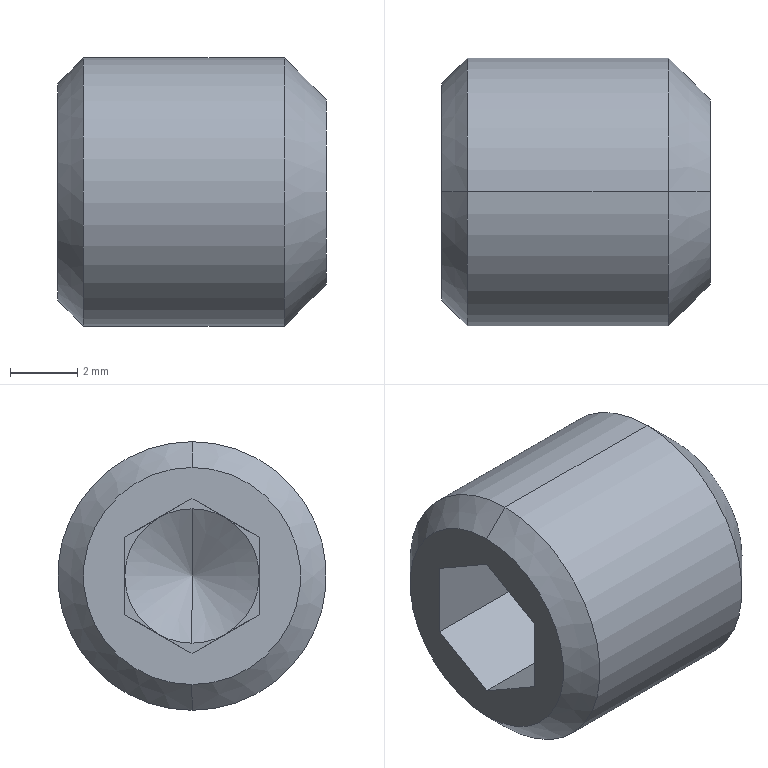Part | STEP file | _SET-SCREW8-8.stp | 1 solid | 22 faces | box 8 x 8 x 8 mm | volume 331.208 mm3 | plane 14 | cone 6 | cylinder 2 | commonest cylinder face diameters 8 x2
STEP:
#1=CARTESIAN_POINT('',(0.,0.,0.));
#2=DIRECTION('',(0.,0.,1.));
#3=DIRECTION('',(1.,0.,0.));
#4=AXIS2_PLACEMENT_3D('',#1,#2,#3);
#5=CARTESIAN_POINT('',(-5.,0.,2.));
#6=VERTEX_POINT('',#5);
#7=CARTESIAN_POINT('',(-5.,-1.,1.732));
#8=VERTEX_POINT('',#7);
#9=CARTESIAN_POINT('',(-5.,0.,0.));
#10=DIRECTION('',(1.,0.,0.));
#11=DIRECTION('',(0.,0.,1.));
#12=AXIS2_PLACEMENT_3D('',#9,#10,#11);
#13=CIRCLE('',#12,2.);
#14=CARTESIAN_POINT('',(-4.845,0.,0.));
#15=DIRECTION('',(-1.,0.,0.));
#16=DIRECTION('',(0.,0.,1.));
#17=AXIS2_PLACEMENT_3D('',#14,#15,#16);
#18=CONICAL_SURFACE('',#17,1.732,1.047);
#19=CARTESIAN_POINT('',(6.283,0.1547));
#20=DIRECTION('',(-1.,0.));
#21=VECTOR('',#20,1.);
#22=LINE('',#19,#21);
#23=(GEOMETRIC_REPRESENTATION_CONTEXT(2)PARAMETRIC_REPRESENTATION_CONTEXT()REPRESENTATION_CONTEXT('',''));
#24=DEFINITIONAL_REPRESENTATION('',(#22),#23);
#25=PCURVE('',#18,#24);
#26=CARTESIAN_POINT('',(-5.,-1.1,1.703));
#27=DIRECTION('',(-1.,0.,0.));
#28=DIRECTION('',(0.,0.,1.));
#29=AXIS2_PLACEMENT_3D('',#26,#27,#28);
#30=PLANE('',#29);
#31=CARTESIAN_POINT('',(0.2968,1.1));
#32=CARTESIAN_POINT('',(0.2968,-2.364));
#33=CARTESIAN_POINT('',(-2.703,-0.6321));
#34=CARTESIAN_POINT('',(-5.703,1.1));
#35=CARTESIAN_POINT('',(-2.703,2.832));
#36=CARTESIAN_POINT('',(0.2968,4.564));
#37=CARTESIAN_POINT('',(0.2968,1.1));
#38=(BOUNDED_CURVE()B_SPLINE_CURVE(2,(#31,#32,#33,#34,#35,#36,#37),.UNSPECIFIED.,.T.,.F.)B_SPLINE_CURVE_WITH_KNOTS((1,2,2,2,2,1),(-2.094,0.,2.094,4.189,6.283,8.378),.UNSPECIFIED.)CURVE()GEOMETRIC_REPRESENTATION_ITEM()RATIONAL_B_SPLINE_CURVE((1.,0.5,1.,0.5,1.,0.5,1.))REPRESENTATION_ITEM(''));
#39=(GEOMETRIC_REPRESENTATION_CONTEXT(2)PARAMETRIC_REPRESENTATION_CONTEXT()REPRESENTATION_CONTEXT('',''));
#40=DEFINITIONAL_REPRESENTATION('',(#38),#39);
#41=PCURVE('',#30,#40);
#42=SURFACE_CURVE('',#13,(#25,#41),.PCURVE_S1.);
#43=EDGE_CURVE('',#6,#8,#42,.T.);
#44=ORIENTED_EDGE('',*,*,#43,.T.);
#45=CARTESIAN_POINT('',(-5.,-2.,0.));
#46=VERTEX_POINT('',#45);
#47=CARTESIAN_POINT('',(-5.,0.,0.));
#48=DIRECTION('',(1.,0.,0.));
#49=DIRECTION('',(0.,0.,1.));
#50=AXIS2_PLACEMENT_3D('',#47,#48,#49);
#51=CIRCLE('',#50,2.);
#52=CARTESIAN_POINT('',(6.283,0.1547));
#53=DIRECTION('',(-1.,0.));
#54=VECTOR('',#53,1.);
#55=LINE('',#52,#54);
#56=(GEOMETRIC_REPRESENTATION_CONTEXT(2)PARAMETRIC_REPRESENTATION_CONTEXT()REPRESENTATION_CONTEXT('',''));
#57=DEFINITIONAL_REPRESENTATION('',(#55),#56);
#58=PCURVE('',#18,#57);
#59=CARTESIAN_POINT('',(-5.,-2.05,-0.0866));
#60=DIRECTION('',(-1.,0.,0.));
#61=DIRECTION('',(0.,0.,1.));
#62=AXIS2_PLACEMENT_3D('',#59,#60,#61);
#63=PLANE('',#62);
#64=CARTESIAN_POINT('',(2.087,2.05));
#65=CARTESIAN_POINT('',(2.087,-1.414));
#66=CARTESIAN_POINT('',(-0.9134,0.3179));
#67=CARTESIAN_POINT('',(-3.913,2.05));
#68=CARTESIAN_POINT('',(-0.9134,3.782));
#69=CARTESIAN_POINT('',(2.087,5.514));
#70=CARTESIAN_POINT('',(2.087,2.05));
#71=(BOUNDED_CURVE()B_SPLINE_CURVE(2,(#64,#65,#66,#67,#68,#69,#70),.UNSPECIFIED.,.T.,.F.)B_SPLINE_CURVE_WITH_KNOTS((1,2,2,2,2,1),(-2.094,0.,2.094,4.189,6.283,8.378),.UNSPECIFIED.)CURVE()GEOMETRIC_REPRESENTATION_ITEM()RATIONAL_B_SPLINE_CURVE((1.,0.5,1.,0.5,1.,0.5,1.))REPRESENTATION_ITEM(''));
#72=(GEOMETRIC_REPRESENTATION_CONTEXT(2)PARAMETRIC_REPRESENTATION_CONTEXT()REPRESENTATION_CONTEXT('',''));
#73=DEFINITIONAL_REPRESENTATION('',(#71),#72);
#74=PCURVE('',#63,#73);
#75=SURFACE_CURVE('',#51,(#58,#74),.PCURVE_S1.);
#76=EDGE_CURVE('',#8,#46,#75,.T.);
#77=ORIENTED_EDGE('',*,*,#76,.T.);
#78=CARTESIAN_POINT('',(-5.,-1.,-1.732));
#79=VERTEX_POINT('',#78);
#80=CARTESIAN_POINT('',(-5.,0.,0.));
#81=DIRECTION('',(1.,0.,0.));
#82=DIRECTION('',(0.,0.,1.));
#83=AXIS2_PLACEMENT_3D('',#80,#81,#82);
#84=CIRCLE('',#83,2.);
#85=CARTESIAN_POINT('',(6.283,0.1547));
#86=DIRECTION('',(-1.,0.));
#87=VECTOR('',#86,1.);
#88=LINE('',#85,#87);
#89=(GEOMETRIC_REPRESENTATION_CONTEXT(2)PARAMETRIC_REPRESENTATION_CONTEXT()REPRESENTATION_CONTEXT('',''));
#90=DEFINITIONAL_REPRESENTATION('',(#88),#89);
#91=PCURVE('',#18,#90);
#92=CARTESIAN_POINT('',(-5.,-2.05,-1.819));
#93=DIRECTION('',(-1.,0.,0.));
#94=DIRECTION('',(0.,0.,1.));
#95=AXIS2_PLACEMENT_3D('',#92,#93,#94);
#96=PLANE('',#95);
#97=CARTESIAN_POINT('',(3.819,2.05));
#98=CARTESIAN_POINT('',(3.819,-1.414));
#99=CARTESIAN_POINT('',(0.8187,0.3179));
#100=CARTESIAN_POINT('',(-2.181,2.05));
#101=CARTESIAN_POINT('',(0.8187,3.782));
#102=CARTESIAN_POINT('',(3.819,5.514));
#103=CARTESIAN_POINT('',(3.819,2.05));
#104=(BOUNDED_CURVE()B_SPLINE_CURVE(2,(#97,#98,#99,#100,#101,#102,#103),.UNSPECIFIED.,.T.,.F.)B_SPLINE_CURVE_WITH_KNOTS((1,2,2,2,2,1),(-2.094,0.,2.094,4.189,6.283,8.378),.UNSPECIFIED.)CURVE()GEOMETRIC_REPRESENTATION_ITEM()RATIONAL_B_SPLINE_CURVE((1.,0.5,1.,0.5,1.,0.5,1.))REPRESENTATION_ITEM(''));
#105=(GEOMETRIC_REPRESENTATION_CONTEXT(2)PARAMETRIC_REPRESENTATION_CONTEXT()REPRESENTATION_CONTEXT('',''));
#106=DEFINITIONAL_REPRESENTATION('',(#104),#105);
#107=PCURVE('',#96,#106);
#108=SURFACE_CURVE('',#84,(#91,#107),.PCURVE_S1.);
#109=EDGE_CURVE('',#46,#79,#108,.T.);
#110=ORIENTED_EDGE('',*,*,#109,.T.);
#111=CARTESIAN_POINT('',(-5.,0.,-2.));
#112=VERTEX_POINT('',#111);
#113=CARTESIAN_POINT('',(-5.,0.,0.));
#114=DIRECTION('',(1.,0.,0.));
#115=DIRECTION('',(0.,0.,1.));
#116=AXIS2_PLACEMENT_3D('',#113,#114,#115);
#117=CIRCLE('',#116,2.);
#118=CARTESIAN_POINT('',(6.283,0.1547));
#119=DIRECTION('',(-1.,0.));
#120=VECTOR('',#119,1.);
#121=LINE('',#118,#120);
#122=(GEOMETRIC_REPRESENTATION_CONTEXT(2)PARAMETRIC_REPRESENTATION_CONTEXT()REPRESENTATION_CONTEXT('',''));
#123=DEFINITIONAL_REPRESENTATION('',(#121),#122);
#124=PCURVE('',#18,#123);
#125=CARTESIAN_POINT('',(-5.,-1.1,-2.338));
#126=DIRECTION('',(-1.,0.,0.));
#127=DIRECTION('',(0.,0.,1.));
#128=AXIS2_PLACEMENT_3D('',#125,#126,#127);
#129=PLANE('',#128);
#130=CARTESIAN_POINT('',(4.338,1.1));
#131=CARTESIAN_POINT('',(4.338,-2.364));
#132=CARTESIAN_POINT('',(1.338,-0.6321));
#133=CARTESIAN_POINT('',(-1.662,1.1));
#134=CARTESIAN_POINT('',(1.338,2.832));
#135=CARTESIAN_POINT('',(4.338,4.564));
#136=CARTESIAN_POINT('',(4.338,1.1));
#137=(BOUNDED_CURVE()B_SPLINE_CURVE(2,(#130,#131,#132,#133,#134,#135,#136),.UNSPECIFIED.,.T.,.F.)B_SPLINE_CURVE_WITH_KNOTS((1,2,2,2,2,1),(-2.094,0.,2.094,4.189,6.283,8.378),.UNSPECIFIED.)CURVE()GEOMETRIC_REPRESENTATION_ITEM()RATIONAL_B_SPLINE_CURVE((1.,0.5,1.,0.5,1.,0.5,1.))REPRESENTATION_ITEM(''));
#138=(GEOMETRIC_REPRESENTATION_CONTEXT(2)PARAMETRIC_REPRESENTATION_CONTEXT()REPRESENTATION_CONTEXT('',''));
#139=DEFINITIONAL_REPRESENTATION('',(#137),#138);
#140=PCURVE('',#129,#139);
#141=SURFACE_CURVE('',#117,(#124,#140),.PCURVE_S1.);
#142=EDGE_CURVE('',#79,#112,#141,.T.);
#143=ORIENTED_EDGE('',*,*,#142,.T.);
#144=CARTESIAN_POINT('',(-3.845,0.,0.));
#145=VERTEX_POINT('',#144);
#146=CARTESIAN_POINT('',(-4.845,0.,-1.732));
#147=DIRECTION('',(-0.5,0.,-0.866));
#148=VECTOR('',#147,1.);
#149=LINE('',#146,#148);
#150=CARTESIAN_POINT('',(3.142,0.));
#151=DIRECTION('',(0.,1.));
#152=VECTOR('',#151,1.);
#153=LINE('',#150,#152);
#154=(GEOMETRIC_REPRESENTATION_CONTEXT(2)PARAMETRIC_REPRESENTATION_CONTEXT()REPRESENTATION_CONTEXT('',''));
#155=DEFINITIONAL_REPRESENTATION('',(#153),#154);
#156=PCURVE('',#18,#155);
#157=CARTESIAN_POINT('',(-4.845,0.,0.));
#158=DIRECTION('',(-1.,0.,0.));
#159=DIRECTION('',(0.,0.,1.));
#160=AXIS2_PLACEMENT_3D('',#157,#158,#159);
#161=CONICAL_SURFACE('',#160,1.732,1.047);
#162=CARTESIAN_POINT('',(3.142,0.));
#163=DIRECTION('',(0.,1.));
#164=VECTOR('',#163,1.);
#165=LINE('',#162,#164);
#166=(GEOMETRIC_REPRESENTATION_CONTEXT(2)PARAMETRIC_REPRESENTATION_CONTEXT()REPRESENTATION_CONTEXT('',''));
#167=DEFINITIONAL_REPRESENTATION('',(#165),#166);
#168=PCURVE('',#161,#167);
#169=SURFACE_CURVE('',#149,(#156,#168),.PCURVE_S1.);
#170=EDGE_CURVE('',#145,#112,#169,.T.);
#171=ORIENTED_EDGE('',*,*,#170,.F.);
#172=CARTESIAN_POINT('',(-4.845,0.,1.732));
#173=DIRECTION('',(-0.5,0.,0.866));
#174=VECTOR('',#173,1.);
#175=LINE('',#172,#174);
#176=CARTESIAN_POINT('',(6.283,0.));
#177=DIRECTION('',(0.,1.));
#178=VECTOR('',#177,1.);
#179=LINE('',#176,#178);
#180=(GEOMETRIC_REPRESENTATION_CONTEXT(2)PARAMETRIC_REPRESENTATION_CONTEXT()REPRESENTATION_CONTEXT('',''));
#181=DEFINITIONAL_REPRESENTATION('',(#179),#180);
#182=PCURVE('',#18,#181);
#183=CARTESIAN_POINT('',(0.,0.));
#184=DIRECTION('',(0.,1.));
#185=VECTOR('',#184,1.);
#186=LINE('',#183,#185);
#187=(GEOMETRIC_REPRESENTATION_CONTEXT(2)PARAMETRIC_REPRESENTATION_CONTEXT()REPRESENTATION_CONTEXT('',''));
#188=DEFINITIONAL_REPRESENTATION('',(#186),#187);
#189=PCURVE('',#161,#188);
#190=SURFACE_CURVE('',#175,(#182,#189),.PCURVE_S1.);
#191=EDGE_CURVE('',#145,#6,#190,.T.);
#192=ORIENTED_EDGE('',*,*,#191,.T.);
#193=EDGE_LOOP('',(#44,#77,#110,#143,#171,#192));
#194=FACE_BOUND('',#193,.F.);
#195=ADVANCED_FACE('',(#194),#18,.F.);
#196=CARTESIAN_POINT('',(-8.,2.,-1.155));
#197=VERTEX_POINT('',#196);
#198=CARTESIAN_POINT('',(-8.,0.,-2.309));
#199=VERTEX_POINT('',#198);
#200=CARTESIAN_POINT('',(-8.,2.,-1.155));
#201=DIRECTION('',(0.,-0.866,-0.5));
#202=VECTOR('',#201,1.);
#203=LINE('',#200,#202);
#204=CARTESIAN_POINT('',(-8.15,-0.1,-2.367));
#205=DIRECTION('',(0.,0.5,-0.866));
#206=DIRECTION('',(-1.,0.,0.));
#207=AXIS2_PLACEMENT_3D('',#204,#205,#206);
#208=PLANE('',#207);
#209=CARTESIAN_POINT('',(-0.15,2.425));
#210=DIRECTION('',(0.,-1.));
#211=VECTOR('',#210,1.);
#212=LINE('',#209,#211);
#213=(GEOMETRIC_REPRESENTATION_CONTEXT(2)PARAMETRIC_REPRESENTATION_CONTEXT()REPRESENTATION_CONTEXT('',''));
#214=DEFINITIONAL_REPRESENTATION('',(#212),#213);
#215=PCURVE('',#208,#214);
#216=CARTESIAN_POINT('',(-8.,-3.556,3.556));
#217=DIRECTION('',(1.,0.,0.));
#218=DIRECTION('',(0.,1.,0.));
#219=AXIS2_PLACEMENT_3D('',#216,#217,#218);
#220=PLANE('',#219);
#221=CARTESIAN_POINT('',(5.556,-4.711));
#222=DIRECTION('',(-0.866,-0.5));
#223=VECTOR('',#222,1.);
#224=LINE('',#221,#223);
#225=(GEOMETRIC_REPRESENTATION_CONTEXT(2)PARAMETRIC_REPRESENTATION_CONTEXT()REPRESENTATION_CONTEXT('',''));
#226=DEFINITIONAL_REPRESENTATION('',(#224),#225);
#227=PCURVE('',#220,#226);
#228=SURFACE_CURVE('',#203,(#215,#227),.PCURVE_S1.);
#229=EDGE_CURVE('',#197,#199,#228,.T.);
#230=ORIENTED_EDGE('',*,*,#229,.T.);
#231=CARTESIAN_POINT('',(-5.,0.,-2.309));
#232=VERTEX_POINT('',#231);
#233=CARTESIAN_POINT('',(-5.,0.,-2.309));
#234=DIRECTION('',(-1.,0.,0.));
#235=VECTOR('',#234,1.);
#236=LINE('',#233,#235);
#237=CARTESIAN_POINT('',(-3.15,0.1155));
#238=DIRECTION('',(1.,0.));
#239=VECTOR('',#238,1.);
#240=LINE('',#237,#239);
#241=(GEOMETRIC_REPRESENTATION_CONTEXT(2)PARAMETRIC_REPRESENTATION_CONTEXT()REPRESENTATION_CONTEXT('',''));
#242=DEFINITIONAL_REPRESENTATION('',(#240),#241);
#243=PCURVE('',#208,#242);
#244=CARTESIAN_POINT('',(-8.15,-2.1,-1.097));
#245=DIRECTION('',(0.,-0.5,-0.866));
#246=DIRECTION('',(0.,-0.866,0.5));
#247=AXIS2_PLACEMENT_3D('',#244,#245,#246);
#248=PLANE('',#247);
#249=CARTESIAN_POINT('',(-2.425,-3.15));
#250=DIRECTION('',(0.,1.));
#251=VECTOR('',#250,1.);
#252=LINE('',#249,#251);
#253=(GEOMETRIC_REPRESENTATION_CONTEXT(2)PARAMETRIC_REPRESENTATION_CONTEXT()REPRESENTATION_CONTEXT('',''));
#254=DEFINITIONAL_REPRESENTATION('',(#252),#253);
#255=PCURVE('',#248,#254);
#256=SURFACE_CURVE('',#236,(#243,#255),.PCURVE_S1.);
#257=EDGE_CURVE('',#232,#199,#256,.T.);
#258=ORIENTED_EDGE('',*,*,#257,.F.);
#259=CARTESIAN_POINT('',(-5.,1.,-1.732));
#260=VERTEX_POINT('',#259);
#261=CARTESIAN_POINT('',(-5.,1.,-1.732));
#262=DIRECTION('',(0.,-0.866,-0.5));
#263=VECTOR('',#262,1.);
#264=LINE('',#261,#263);
#265=CARTESIAN_POINT('',(-3.15,1.27));
#266=DIRECTION('',(0.,-1.));
#267=VECTOR('',#266,1.);
#268=LINE('',#265,#267);
#269=(GEOMETRIC_REPRESENTATION_CONTEXT(2)PARAMETRIC_REPRESENTATION_CONTEXT()REPRESENTATION_CONTEXT('',''));
#270=DEFINITIONAL_REPRESENTATION('',(#268),#269);
#271=PCURVE('',#208,#270);
#272=CARTESIAN_POINT('',(0.6062,2.1));
#273=DIRECTION('',(-0.5,-0.866));
#274=VECTOR('',#273,1.);
#275=LINE('',#272,#274);
#276=(GEOMETRIC_REPRESENTATION_CONTEXT(2)PARAMETRIC_REPRESENTATION_CONTEXT()REPRESENTATION_CONTEXT('',''));
#277=DEFINITIONAL_REPRESENTATION('',(#275),#276);
#278=PCURVE('',#129,#277);
#279=SURFACE_CURVE('',#264,(#271,#278),.PCURVE_S1.);
#280=EDGE_CURVE('',#260,#232,#279,.T.);
#281=ORIENTED_EDGE('',*,*,#280,.F.);
#282=CARTESIAN_POINT('',(-5.,2.,-1.155));
#283=VERTEX_POINT('',#282);
#284=CARTESIAN_POINT('',(-5.,2.,-1.155));
#285=DIRECTION('',(0.,-0.866,-0.5));
#286=VECTOR('',#285,1.);
#287=LINE('',#284,#286);
#288=CARTESIAN_POINT('',(-3.15,2.425));
#289=DIRECTION('',(0.,-1.));
#290=VECTOR('',#289,1.);
#291=LINE('',#288,#290);
#292=(GEOMETRIC_REPRESENTATION_CONTEXT(2)PARAMETRIC_REPRESENTATION_CONTEXT()REPRESENTATION_CONTEXT('',''));
#293=DEFINITIONAL_REPRESENTATION('',(#291),#292);
#294=PCURVE('',#208,#293);
#295=CARTESIAN_POINT('',(-5.,0.95,-1.819));
#296=DIRECTION('',(-1.,0.,0.));
#297=DIRECTION('',(0.,0.,1.));
#298=AXIS2_PLACEMENT_3D('',#295,#296,#297);
#299=PLANE('',#298);
#300=CARTESIAN_POINT('',(0.664,1.05));
#301=DIRECTION('',(-0.5,-0.866));
#302=VECTOR('',#301,1.);
#303=LINE('',#300,#302);
#304=(GEOMETRIC_REPRESENTATION_CONTEXT(2)PARAMETRIC_REPRESENTATION_CONTEXT()REPRESENTATION_CONTEXT('',''));
#305=DEFINITIONAL_REPRESENTATION('',(#303),#304);
#306=PCURVE('',#299,#305);
#307=SURFACE_CURVE('',#287,(#294,#306),.PCURVE_S1.);
#308=EDGE_CURVE('',#283,#260,#307,.T.);
#309=ORIENTED_EDGE('',*,*,#308,.F.);
#310=CARTESIAN_POINT('',(-5.,2.,-1.155));
#311=DIRECTION('',(-1.,0.,0.));
#312=VECTOR('',#311,1.);
#313=LINE('',#310,#312);
#314=CARTESIAN_POINT('',(-3.15,2.425));
#315=DIRECTION('',(1.,0.));
#316=VECTOR('',#315,1.);
#317=LINE('',#314,#316);
#318=(GEOMETRIC_REPRESENTATION_CONTEXT(2)PARAMETRIC_REPRESENTATION_CONTEXT()REPRESENTATION_CONTEXT('',''));
#319=DEFINITIONAL_REPRESENTATION('',(#317),#318);
#320=PCURVE('',#208,#319);
#321=CARTESIAN_POINT('',(-8.15,2.,-1.27));
#322=DIRECTION('',(0.,1.,0.));
#323=DIRECTION('',(1.,0.,0.));
#324=AXIS2_PLACEMENT_3D('',#321,#322,#323);
#325=PLANE('',#324);
#326=CARTESIAN_POINT('',(3.15,-0.1155));
#327=DIRECTION('',(-1.,0.));
#328=VECTOR('',#327,1.);
#329=LINE('',#326,#328);
#330=(GEOMETRIC_REPRESENTATION_CONTEXT(2)PARAMETRIC_REPRESENTATION_CONTEXT()REPRESENTATION_CONTEXT('',''));
#331=DEFINITIONAL_REPRESENTATION('',(#329),#330);
#332=PCURVE('',#325,#331);
#333=SURFACE_CURVE('',#313,(#320,#332),.PCURVE_S1.);
#334=EDGE_CURVE('',#283,#197,#333,.T.);
#335=ORIENTED_EDGE('',*,*,#334,.T.);
#336=EDGE_LOOP('',(#230,#258,#281,#309,#335));
#337=FACE_BOUND('',#336,.T.);
#338=ADVANCED_FACE('',(#337),#208,.F.);
#339=CARTESIAN_POINT('',(-5.,2.,1.155));
#340=VERTEX_POINT('',#339);
#341=CARTESIAN_POINT('',(-8.,2.,1.155));
#342=VERTEX_POINT('',#341);
#343=CARTESIAN_POINT('',(-5.,2.,1.155));
#344=DIRECTION('',(-1.,0.,0.));
#345=VECTOR('',#344,1.);
#346=LINE('',#343,#345);
#347=CARTESIAN_POINT('',(3.15,-2.425));
#348=DIRECTION('',(-1.,0.));
#349=VECTOR('',#348,1.);
#350=LINE('',#347,#349);
#351=(GEOMETRIC_REPRESENTATION_CONTEXT(2)PARAMETRIC_REPRESENTATION_CONTEXT()REPRESENTATION_CONTEXT('',''));
#352=DEFINITIONAL_REPRESENTATION('',(#350),#351);
#353=PCURVE('',#325,#352);
#354=CARTESIAN_POINT('',(-8.15,2.1,1.097));
#355=DIRECTION('',(0.,0.5,0.866));
#356=DIRECTION('',(1.,0.,0.));
#357=AXIS2_PLACEMENT_3D('',#354,#355,#356);
#358=PLANE('',#357);
#359=CARTESIAN_POINT('',(3.15,-0.1155));
#360=DIRECTION('',(-1.,0.));
#361=VECTOR('',#360,1.);
#362=LINE('',#359,#361);
#363=(GEOMETRIC_REPRESENTATION_CONTEXT(2)PARAMETRIC_REPRESENTATION_CONTEXT()REPRESENTATION_CONTEXT('',''));
#364=DEFINITIONAL_REPRESENTATION('',(#362),#363);
#365=PCURVE('',#358,#364);
#366=SURFACE_CURVE('',#346,(#353,#365),.PCURVE_S1.);
#367=EDGE_CURVE('',#340,#342,#366,.T.);
#368=ORIENTED_EDGE('',*,*,#367,.T.);
#369=CARTESIAN_POINT('',(-8.,2.,-1.155));
#370=DIRECTION('',(0.,0.,1.));
#371=VECTOR('',#370,1.);
#372=LINE('',#369,#371);
#373=CARTESIAN_POINT('',(0.15,-0.1155));
#374=DIRECTION('',(0.,-1.));
#375=VECTOR('',#374,1.);
#376=LINE('',#373,#375);
#377=(GEOMETRIC_REPRESENTATION_CONTEXT(2)PARAMETRIC_REPRESENTATION_CONTEXT()REPRESENTATION_CONTEXT('',''));
#378=DEFINITIONAL_REPRESENTATION('',(#376),#377);
#379=PCURVE('',#325,#378);
#380=CARTESIAN_POINT('',(5.556,-4.711));
#381=DIRECTION('',(0.,1.));
#382=VECTOR('',#381,1.);
#383=LINE('',#380,#382);
#384=(GEOMETRIC_REPRESENTATION_CONTEXT(2)PARAMETRIC_REPRESENTATION_CONTEXT()REPRESENTATION_CONTEXT('',''));
#385=DEFINITIONAL_REPRESENTATION('',(#383),#384);
#386=PCURVE('',#220,#385);
#387=SURFACE_CURVE('',#372,(#379,#386),.PCURVE_S1.);
#388=EDGE_CURVE('',#197,#342,#387,.T.);
#389=ORIENTED_EDGE('',*,*,#388,.F.);
#390=ORIENTED_EDGE('',*,*,#334,.F.);
#391=CARTESIAN_POINT('',(-5.,2.,0.));
#392=VERTEX_POINT('',#391);
#393=CARTESIAN_POINT('',(-5.,2.,0.));
#394=DIRECTION('',(0.,0.,-1.));
#395=VECTOR('',#394,1.);
#396=LINE('',#393,#395);
#397=CARTESIAN_POINT('',(3.15,-1.27));
#398=DIRECTION('',(0.,1.));
#399=VECTOR('',#398,1.);
#400=LINE('',#397,#399);
#401=(GEOMETRIC_REPRESENTATION_CONTEXT(2)PARAMETRIC_REPRESENTATION_CONTEXT()REPRESENTATION_CONTEXT('',''));
#402=DEFINITIONAL_REPRESENTATION('',(#400),#401);
#403=PCURVE('',#325,#402);
#404=CARTESIAN_POINT('',(1.819,1.05));
#405=DIRECTION('',(-1.,0.));
#406=VECTOR('',#405,1.);
#407=LINE('',#404,#406);
#408=(GEOMETRIC_REPRESENTATION_CONTEXT(2)PARAMETRIC_REPRESENTATION_CONTEXT()REPRESENTATION_CONTEXT('',''));
#409=DEFINITIONAL_REPRESENTATION('',(#407),#408);
#410=PCURVE('',#299,#409);
#411=SURFACE_CURVE('',#396,(#403,#410),.PCURVE_S1.);
#412=EDGE_CURVE('',#392,#283,#411,.T.);
#413=ORIENTED_EDGE('',*,*,#412,.F.);
#414=CARTESIAN_POINT('',(-5.,2.,1.155));
#415=DIRECTION('',(0.,0.,-1.));
#416=VECTOR('',#415,1.);
#417=LINE('',#414,#416);
#418=CARTESIAN_POINT('',(3.15,-2.425));
#419=DIRECTION('',(0.,1.));
#420=VECTOR('',#419,1.);
#421=LINE('',#418,#420);
#422=(GEOMETRIC_REPRESENTATION_CONTEXT(2)PARAMETRIC_REPRESENTATION_CONTEXT()REPRESENTATION_CONTEXT('',''));
#423=DEFINITIONAL_REPRESENTATION('',(#421),#422);
#424=PCURVE('',#325,#423);
#425=CARTESIAN_POINT('',(-5.,0.95,-0.0866));
#426=DIRECTION('',(-1.,0.,0.));
#427=DIRECTION('',(0.,0.,1.));
#428=AXIS2_PLACEMENT_3D('',#425,#426,#427);
#429=PLANE('',#428);
#430=CARTESIAN_POINT('',(1.241,1.05));
#431=DIRECTION('',(-1.,0.));
#432=VECTOR('',#431,1.);
#433=LINE('',#430,#432);
#434=(GEOMETRIC_REPRESENTATION_CONTEXT(2)PARAMETRIC_REPRESENTATION_CONTEXT()REPRESENTATION_CONTEXT('',''));
#435=DEFINITIONAL_REPRESENTATION('',(#433),#434);
#436=PCURVE('',#429,#435);
#437=SURFACE_CURVE('',#417,(#424,#436),.PCURVE_S1.);
#438=EDGE_CURVE('',#340,#392,#437,.T.);
#439=ORIENTED_EDGE('',*,*,#438,.F.);
#440=EDGE_LOOP('',(#368,#389,#390,#413,#439));
#441=FACE_BOUND('',#440,.T.);
#442=ADVANCED_FACE('',(#441),#325,.F.);
#443=CARTESIAN_POINT('',(-8.,0.,2.309));
#444=VERTEX_POINT('',#443);
#445=CARTESIAN_POINT('',(-8.,0.,2.309));
#446=DIRECTION('',(0.,0.866,-0.5));
#447=VECTOR('',#446,1.);
#448=LINE('',#445,#447);
#449=CARTESIAN_POINT('',(0.15,-2.425));
#450=DIRECTION('',(0.,1.));
#451=VECTOR('',#450,1.);
#452=LINE('',#449,#451);
#453=(GEOMETRIC_REPRESENTATION_CONTEXT(2)PARAMETRIC_REPRESENTATION_CONTEXT()REPRESENTATION_CONTEXT('',''));
#454=DEFINITIONAL_REPRESENTATION('',(#452),#453);
#455=PCURVE('',#358,#454);
#456=CARTESIAN_POINT('',(3.556,-1.247));
#457=DIRECTION('',(0.866,-0.5));
#458=VECTOR('',#457,1.);
#459=LINE('',#456,#458);
#460=(GEOMETRIC_REPRESENTATION_CONTEXT(2)PARAMETRIC_REPRESENTATION_CONTEXT()REPRESENTATION_CONTEXT('',''));
#461=DEFINITIONAL_REPRESENTATION('',(#459),#460);
#462=PCURVE('',#220,#461);
#463=SURFACE_CURVE('',#448,(#455,#462),.PCURVE_S1.);
#464=EDGE_CURVE('',#444,#342,#463,.T.);
#465=ORIENTED_EDGE('',*,*,#464,.T.);
#466=ORIENTED_EDGE('',*,*,#367,.F.);
#467=CARTESIAN_POINT('',(-5.,1.,1.732));
#468=VERTEX_POINT('',#467);
#469=CARTESIAN_POINT('',(-5.,1.,1.732));
#470=DIRECTION('',(0.,0.866,-0.5));
#471=VECTOR('',#470,1.);
#472=LINE('',#469,#471);
#473=CARTESIAN_POINT('',(3.15,-1.27));
#474=DIRECTION('',(0.,1.));
#475=VECTOR('',#474,1.);
#476=LINE('',#473,#475);
#477=(GEOMETRIC_REPRESENTATION_CONTEXT(2)PARAMETRIC_REPRESENTATION_CONTEXT()REPRESENTATION_CONTEXT('',''));
#478=DEFINITIONAL_REPRESENTATION('',(#476),#477);
#479=PCURVE('',#358,#478);
#480=CARTESIAN_POINT('',(1.819,0.05));
#481=DIRECTION('',(-0.5,0.866));
#482=VECTOR('',#481,1.);
#483=LINE('',#480,#482);
#484=(GEOMETRIC_REPRESENTATION_CONTEXT(2)PARAMETRIC_REPRESENTATION_CONTEXT()REPRESENTATION_CONTEXT('',''));
#485=DEFINITIONAL_REPRESENTATION('',(#483),#484);
#486=PCURVE('',#429,#485);
#487=SURFACE_CURVE('',#472,(#479,#486),.PCURVE_S1.);
#488=EDGE_CURVE('',#468,#340,#487,.T.);
#489=ORIENTED_EDGE('',*,*,#488,.F.);
#490=CARTESIAN_POINT('',(-5.,0.,2.309));
#491=VERTEX_POINT('',#490);
#492=CARTESIAN_POINT('',(-5.,0.,2.309));
#493=DIRECTION('',(0.,0.866,-0.5));
#494=VECTOR('',#493,1.);
#495=LINE('',#492,#494);
#496=CARTESIAN_POINT('',(3.15,-2.425));
#497=DIRECTION('',(0.,1.));
#498=VECTOR('',#497,1.);
#499=LINE('',#496,#498);
#500=(GEOMETRIC_REPRESENTATION_CONTEXT(2)PARAMETRIC_REPRESENTATION_CONTEXT()REPRESENTATION_CONTEXT('',''));
#501=DEFINITIONAL_REPRESENTATION('',(#499),#500);
#502=PCURVE('',#358,#501);
#503=CARTESIAN_POINT('',(0.6062,1.1));
#504=DIRECTION('',(-0.5,0.866));
#505=VECTOR('',#504,1.);
#506=LINE('',#503,#505);
#507=(GEOMETRIC_REPRESENTATION_CONTEXT(2)PARAMETRIC_REPRESENTATION_CONTEXT()REPRESENTATION_CONTEXT('',''));
#508=DEFINITIONAL_REPRESENTATION('',(#506),#507);
#509=PCURVE('',#30,#508);
#510=SURFACE_CURVE('',#495,(#502,#509),.PCURVE_S1.);
#511=EDGE_CURVE('',#491,#468,#510,.T.);
#512=ORIENTED_EDGE('',*,*,#511,.F.);
#513=CARTESIAN_POINT('',(-5.,0.,2.309));
#514=DIRECTION('',(-1.,0.,0.));
#515=VECTOR('',#514,1.);
#516=LINE('',#513,#515);
#517=CARTESIAN_POINT('',(3.15,-2.425));
#518=DIRECTION('',(-1.,0.));
#519=VECTOR('',#518,1.);
#520=LINE('',#517,#519);
#521=(GEOMETRIC_REPRESENTATION_CONTEXT(2)PARAMETRIC_REPRESENTATION_CONTEXT()REPRESENTATION_CONTEXT('',''));
#522=DEFINITIONAL_REPRESENTATION('',(#520),#521);
#523=PCURVE('',#358,#522);
#524=CARTESIAN_POINT('',(-8.15,0.1,2.367));
#525=DIRECTION('',(0.,-0.5,0.866));
#526=DIRECTION('',(-1.,0.,0.));
#527=AXIS2_PLACEMENT_3D('',#524,#525,#526);
#528=PLANE('',#527);
#529=CARTESIAN_POINT('',(-3.15,0.1155));
#530=DIRECTION('',(1.,0.));
#531=VECTOR('',#530,1.);
#532=LINE('',#529,#531);
#533=(GEOMETRIC_REPRESENTATION_CONTEXT(2)PARAMETRIC_REPRESENTATION_CONTEXT()REPRESENTATION_CONTEXT('',''));
#534=DEFINITIONAL_REPRESENTATION('',(#532),#533);
#535=PCURVE('',#528,#534);
#536=SURFACE_CURVE('',#516,(#523,#535),.PCURVE_S1.);
#537=EDGE_CURVE('',#491,#444,#536,.T.);
#538=ORIENTED_EDGE('',*,*,#537,.T.);
#539=EDGE_LOOP('',(#465,#466,#489,#512,#538));
#540=FACE_BOUND('',#539,.T.);
#541=ADVANCED_FACE('',(#540),#358,.F.);
#542=CARTESIAN_POINT('',(-8.,-2.,1.155));
#543=VERTEX_POINT('',#542);
#544=CARTESIAN_POINT('',(-8.,-2.,1.155));
#545=DIRECTION('',(0.,0.866,0.5));
#546=VECTOR('',#545,1.);
#547=LINE('',#544,#546);
#548=CARTESIAN_POINT('',(-0.15,2.425));
#549=DIRECTION('',(0.,-1.));
#550=VECTOR('',#549,1.);
#551=LINE('',#548,#550);
#552=(GEOMETRIC_REPRESENTATION_CONTEXT(2)PARAMETRIC_REPRESENTATION_CONTEXT()REPRESENTATION_CONTEXT('',''));
#553=DEFINITIONAL_REPRESENTATION('',(#551),#552);
#554=PCURVE('',#528,#553);
#555=CARTESIAN_POINT('',(1.556,-2.402));
#556=DIRECTION('',(0.866,0.5));
#557=VECTOR('',#556,1.);
#558=LINE('',#555,#557);
#559=(GEOMETRIC_REPRESENTATION_CONTEXT(2)PARAMETRIC_REPRESENTATION_CONTEXT()REPRESENTATION_CONTEXT('',''));
#560=DEFINITIONAL_REPRESENTATION('',(#558),#559);
#561=PCURVE('',#220,#560);
#562=SURFACE_CURVE('',#547,(#554,#561),.PCURVE_S1.);
#563=EDGE_CURVE('',#543,#444,#562,.T.);
#564=ORIENTED_EDGE('',*,*,#563,.T.);
#565=ORIENTED_EDGE('',*,*,#537,.F.);
#566=CARTESIAN_POINT('',(-5.,-1.,1.732));
#567=DIRECTION('',(0.,0.866,0.5));
#568=VECTOR('',#567,1.);
#569=LINE('',#566,#568);
#570=CARTESIAN_POINT('',(-3.15,1.27));
#571=DIRECTION('',(0.,-1.));
#572=VECTOR('',#571,1.);
#573=LINE('',#570,#572);
#574=(GEOMETRIC_REPRESENTATION_CONTEXT(2)PARAMETRIC_REPRESENTATION_CONTEXT()REPRESENTATION_CONTEXT('',''));
#575=DEFINITIONAL_REPRESENTATION('',(#573),#574);
#576=PCURVE('',#528,#575);
#577=CARTESIAN_POINT('',(0.02887,0.1));
#578=DIRECTION('',(0.5,0.866));
#579=VECTOR('',#578,1.);
#580=LINE('',#577,#579);
#581=(GEOMETRIC_REPRESENTATION_CONTEXT(2)PARAMETRIC_REPRESENTATION_CONTEXT()REPRESENTATION_CONTEXT('',''));
#582=DEFINITIONAL_REPRESENTATION('',(#580),#581);
#583=PCURVE('',#30,#582);
#584=SURFACE_CURVE('',#569,(#576,#583),.PCURVE_S1.);
#585=EDGE_CURVE('',#8,#491,#584,.T.);
#586=ORIENTED_EDGE('',*,*,#585,.F.);
#587=CARTESIAN_POINT('',(-5.,-2.,1.155));
#588=VERTEX_POINT('',#587);
#589=CARTESIAN_POINT('',(-5.,-2.,1.155));
#590=DIRECTION('',(0.,0.866,0.5));
#591=VECTOR('',#590,1.);
#592=LINE('',#589,#591);
#593=CARTESIAN_POINT('',(-3.15,2.425));
#594=DIRECTION('',(0.,-1.));
#595=VECTOR('',#594,1.);
#596=LINE('',#593,#595);
#597=(GEOMETRIC_REPRESENTATION_CONTEXT(2)PARAMETRIC_REPRESENTATION_CONTEXT()REPRESENTATION_CONTEXT('',''));
#598=DEFINITIONAL_REPRESENTATION('',(#596),#597);
#599=PCURVE('',#528,#598);
#600=CARTESIAN_POINT('',(1.241,0.05));
#601=DIRECTION('',(0.5,0.866));
#602=VECTOR('',#601,1.);
#603=LINE('',#600,#602);
#604=(GEOMETRIC_REPRESENTATION_CONTEXT(2)PARAMETRIC_REPRESENTATION_CONTEXT()REPRESENTATION_CONTEXT('',''));
#605=DEFINITIONAL_REPRESENTATION('',(#603),#604);
#606=PCURVE('',#63,#605);
#607=SURFACE_CURVE('',#592,(#599,#606),.PCURVE_S1.);
#608=EDGE_CURVE('',#588,#8,#607,.T.);
#609=ORIENTED_EDGE('',*,*,#608,.F.);
#610=CARTESIAN_POINT('',(-5.,-2.,1.155));
#611=DIRECTION('',(-1.,0.,0.));
#612=VECTOR('',#611,1.);
#613=LINE('',#610,#612);
#614=CARTESIAN_POINT('',(-3.15,2.425));
#615=DIRECTION('',(1.,0.));
#616=VECTOR('',#615,1.);
#617=LINE('',#614,#616);
#618=(GEOMETRIC_REPRESENTATION_CONTEXT(2)PARAMETRIC_REPRESENTATION_CONTEXT()REPRESENTATION_CONTEXT('',''));
#619=DEFINITIONAL_REPRESENTATION('',(#617),#618);
#620=PCURVE('',#528,#619);
#621=CARTESIAN_POINT('',(-8.15,-2.,1.27));
#622=DIRECTION('',(0.,-1.,0.));
#623=DIRECTION('',(0.,0.,-1.));
#624=AXIS2_PLACEMENT_3D('',#621,#622,#623);
#625=PLANE('',#624);
#626=CARTESIAN_POINT('',(0.1155,3.15));
#627=DIRECTION('',(0.,-1.));
#628=VECTOR('',#627,1.);
#629=LINE('',#626,#628);
#630=(GEOMETRIC_REPRESENTATION_CONTEXT(2)PARAMETRIC_REPRESENTATION_CONTEXT()REPRESENTATION_CONTEXT('',''));
#631=DEFINITIONAL_REPRESENTATION('',(#629),#630);
#632=PCURVE('',#625,#631);
#633=SURFACE_CURVE('',#613,(#620,#632),.PCURVE_S1.);
#634=EDGE_CURVE('',#588,#543,#633,.T.);
#635=ORIENTED_EDGE('',*,*,#634,.T.);
#636=EDGE_LOOP('',(#564,#565,#586,#609,#635));
#637=FACE_BOUND('',#636,.T.);
#638=ADVANCED_FACE('',(#637),#528,.F.);
#639=CARTESIAN_POINT('',(-8.,-2.,-1.155));
#640=VERTEX_POINT('',#639);
#641=CARTESIAN_POINT('',(-8.,-2.,-1.155));
#642=DIRECTION('',(0.,0.,1.));
#643=VECTOR('',#642,1.);
#644=LINE('',#641,#643);
#645=CARTESIAN_POINT('',(2.425,0.15));
#646=DIRECTION('',(-1.,0.));
#647=VECTOR('',#646,1.);
#648=LINE('',#645,#647);
#649=(GEOMETRIC_REPRESENTATION_CONTEXT(2)PARAMETRIC_REPRESENTATION_CONTEXT()REPRESENTATION_CONTEXT('',''));
#650=DEFINITIONAL_REPRESENTATION('',(#648),#649);
#651=PCURVE('',#625,#650);
#652=CARTESIAN_POINT('',(1.556,-4.711));
#653=DIRECTION('',(0.,1.));
#654=VECTOR('',#653,1.);
#655=LINE('',#652,#654);
#656=(GEOMETRIC_REPRESENTATION_CONTEXT(2)PARAMETRIC_REPRESENTATION_CONTEXT()REPRESENTATION_CONTEXT('',''));
#657=DEFINITIONAL_REPRESENTATION('',(#655),#656);
#658=PCURVE('',#220,#657);
#659=SURFACE_CURVE('',#644,(#651,#658),.PCURVE_S1.);
#660=EDGE_CURVE('',#640,#543,#659,.T.);
#661=ORIENTED_EDGE('',*,*,#660,.T.);
#662=ORIENTED_EDGE('',*,*,#634,.F.);
#663=CARTESIAN_POINT('',(-5.,-2.,0.));
#664=DIRECTION('',(0.,0.,1.));
#665=VECTOR('',#664,1.);
#666=LINE('',#663,#665);
#667=CARTESIAN_POINT('',(1.27,3.15));
#668=DIRECTION('',(-1.,0.));
#669=VECTOR('',#668,1.);
#670=LINE('',#667,#669);
#671=(GEOMETRIC_REPRESENTATION_CONTEXT(2)PARAMETRIC_REPRESENTATION_CONTEXT()REPRESENTATION_CONTEXT('',''));
#672=DEFINITIONAL_REPRESENTATION('',(#670),#671);
#673=PCURVE('',#625,#672);
#674=CARTESIAN_POINT('',(0.0866,0.05));
#675=DIRECTION('',(1.,0.));
#676=VECTOR('',#675,1.);
#677=LINE('',#674,#676);
#678=(GEOMETRIC_REPRESENTATION_CONTEXT(2)PARAMETRIC_REPRESENTATION_CONTEXT()REPRESENTATION_CONTEXT('',''));
#679=DEFINITIONAL_REPRESENTATION('',(#677),#678);
#680=PCURVE('',#63,#679);
#681=SURFACE_CURVE('',#666,(#673,#680),.PCURVE_S1.);
#682=EDGE_CURVE('',#46,#588,#681,.T.);
#683=ORIENTED_EDGE('',*,*,#682,.F.);
#684=CARTESIAN_POINT('',(-5.,-2.,-1.155));
#685=VERTEX_POINT('',#684);
#686=CARTESIAN_POINT('',(-5.,-2.,-1.155));
#687=DIRECTION('',(0.,0.,1.));
#688=VECTOR('',#687,1.);
#689=LINE('',#686,#688);
#690=CARTESIAN_POINT('',(2.425,3.15));
#691=DIRECTION('',(-1.,0.));
#692=VECTOR('',#691,1.);
#693=LINE('',#690,#692);
#694=(GEOMETRIC_REPRESENTATION_CONTEXT(2)PARAMETRIC_REPRESENTATION_CONTEXT()REPRESENTATION_CONTEXT('',''));
#695=DEFINITIONAL_REPRESENTATION('',(#693),#694);
#696=PCURVE('',#625,#695);
#697=CARTESIAN_POINT('',(0.664,0.05));
#698=DIRECTION('',(1.,0.));
#699=VECTOR('',#698,1.);
#700=LINE('',#697,#699);
#701=(GEOMETRIC_REPRESENTATION_CONTEXT(2)PARAMETRIC_REPRESENTATION_CONTEXT()REPRESENTATION_CONTEXT('',''));
#702=DEFINITIONAL_REPRESENTATION('',(#700),#701);
#703=PCURVE('',#96,#702);
#704=SURFACE_CURVE('',#689,(#696,#703),.PCURVE_S1.);
#705=EDGE_CURVE('',#685,#46,#704,.T.);
#706=ORIENTED_EDGE('',*,*,#705,.F.);
#707=CARTESIAN_POINT('',(-5.,-2.,-1.155));
#708=DIRECTION('',(-1.,0.,0.));
#709=VECTOR('',#708,1.);
#710=LINE('',#707,#709);
#711=CARTESIAN_POINT('',(2.425,3.15));
#712=DIRECTION('',(0.,-1.));
#713=VECTOR('',#712,1.);
#714=LINE('',#711,#713);
#715=(GEOMETRIC_REPRESENTATION_CONTEXT(2)PARAMETRIC_REPRESENTATION_CONTEXT()REPRESENTATION_CONTEXT('',''));
#716=DEFINITIONAL_REPRESENTATION('',(#714),#715);
#717=PCURVE('',#625,#716);
#718=CARTESIAN_POINT('',(-0.1155,-3.15));
#719=DIRECTION('',(0.,1.));
#720=VECTOR('',#719,1.);
#721=LINE('',#718,#720);
#722=(GEOMETRIC_REPRESENTATION_CONTEXT(2)PARAMETRIC_REPRESENTATION_CONTEXT()REPRESENTATION_CONTEXT('',''));
#723=DEFINITIONAL_REPRESENTATION('',(#721),#722);
#724=PCURVE('',#248,#723);
#725=SURFACE_CURVE('',#710,(#717,#724),.PCURVE_S1.);
#726=EDGE_CURVE('',#685,#640,#725,.T.);
#727=ORIENTED_EDGE('',*,*,#726,.T.);
#728=EDGE_LOOP('',(#661,#662,#683,#706,#727));
#729=FACE_BOUND('',#728,.T.);
#730=ADVANCED_FACE('',(#729),#625,.F.);
#731=CARTESIAN_POINT('',(0.,0.,-2.75));
#732=VERTEX_POINT('',#731);
#733=CARTESIAN_POINT('',(0.,0.,2.75));
#734=VERTEX_POINT('',#733);
#735=CARTESIAN_POINT('',(0.,0.,0.));
#736=DIRECTION('',(1.,0.,0.));
#737=DIRECTION('',(0.,0.,-1.));
#738=AXIS2_PLACEMENT_3D('',#735,#736,#737);
#739=CIRCLE('',#738,2.75);
#740=CARTESIAN_POINT('',(0.,-3.025,-3.025));
#741=DIRECTION('',(-1.,0.,0.));
#742=DIRECTION('',(0.,0.,1.));
#743=AXIS2_PLACEMENT_3D('',#740,#741,#742);
#744=PLANE('',#743);
#745=CARTESIAN_POINT('',(0.275,3.025));
#746=CARTESIAN_POINT('',(0.275,7.788));
#747=CARTESIAN_POINT('',(4.4,5.407));
#748=CARTESIAN_POINT('',(8.525,3.025));
#749=CARTESIAN_POINT('',(4.4,0.6434));
#750=CARTESIAN_POINT('',(0.275,-1.738));
#751=CARTESIAN_POINT('',(0.275,3.025));
#752=(BOUNDED_CURVE()B_SPLINE_CURVE(2,(#745,#746,#747,#748,#749,#750,#751),.UNSPECIFIED.,.T.,.F.)B_SPLINE_CURVE_WITH_KNOTS((1,2,2,2,2,1),(-2.094,0.,2.094,4.189,6.283,8.378),.UNSPECIFIED.)CURVE()GEOMETRIC_REPRESENTATION_ITEM()RATIONAL_B_SPLINE_CURVE((1.,0.5,1.,0.5,1.,0.5,1.))REPRESENTATION_ITEM(''));
#753=(GEOMETRIC_REPRESENTATION_CONTEXT(2)PARAMETRIC_REPRESENTATION_CONTEXT()REPRESENTATION_CONTEXT('',''));
#754=DEFINITIONAL_REPRESENTATION('',(#752),#753);
#755=PCURVE('',#744,#754);
#756=CARTESIAN_POINT('',(0.0625,0.,0.));
#757=DIRECTION('',(-1.,0.,0.));
#758=DIRECTION('',(0.,0.,1.));
#759=AXIS2_PLACEMENT_3D('',#756,#757,#758);
#760=CONICAL_SURFACE('',#759,2.687,0.7854);
#761=CARTESIAN_POINT('',(3.142,0.0625));
#762=DIRECTION('',(-1.,0.));
#763=VECTOR('',#762,1.);
#764=LINE('',#761,#763);
#765=(GEOMETRIC_REPRESENTATION_CONTEXT(2)PARAMETRIC_REPRESENTATION_CONTEXT()REPRESENTATION_CONTEXT('',''));
#766=DEFINITIONAL_REPRESENTATION('',(#764),#765);
#767=PCURVE('',#760,#766);
#768=SURFACE_CURVE('',#739,(#755,#767),.PCURVE_S1.);
#769=EDGE_CURVE('',#732,#734,#768,.T.);
#770=ORIENTED_EDGE('',*,*,#769,.T.);
#771=CARTESIAN_POINT('',(0.,0.,0.));
#772=DIRECTION('',(1.,0.,0.));
#773=DIRECTION('',(0.,0.,-1.));
#774=AXIS2_PLACEMENT_3D('',#771,#772,#773);
#775=CIRCLE('',#774,2.75);
#776=CARTESIAN_POINT('',(0.275,3.025));
#777=CARTESIAN_POINT('',(0.275,7.788));
#778=CARTESIAN_POINT('',(4.4,5.407));
#779=CARTESIAN_POINT('',(8.525,3.025));
#780=CARTESIAN_POINT('',(4.4,0.6434));
#781=CARTESIAN_POINT('',(0.275,-1.738));
#782=CARTESIAN_POINT('',(0.275,3.025));
#783=(BOUNDED_CURVE()B_SPLINE_CURVE(2,(#776,#777,#778,#779,#780,#781,#782),.UNSPECIFIED.,.T.,.F.)B_SPLINE_CURVE_WITH_KNOTS((1,2,2,2,2,1),(-2.094,0.,2.094,4.189,6.283,8.378),.UNSPECIFIED.)CURVE()GEOMETRIC_REPRESENTATION_ITEM()RATIONAL_B_SPLINE_CURVE((1.,0.5,1.,0.5,1.,0.5,1.))REPRESENTATION_ITEM(''));
#784=(GEOMETRIC_REPRESENTATION_CONTEXT(2)PARAMETRIC_REPRESENTATION_CONTEXT()REPRESENTATION_CONTEXT('',''));
#785=DEFINITIONAL_REPRESENTATION('',(#783),#784);
#786=PCURVE('',#744,#785);
#787=CARTESIAN_POINT('',(0.0625,0.,0.));
#788=DIRECTION('',(-1.,0.,0.));
#789=DIRECTION('',(0.,0.,1.));
#790=AXIS2_PLACEMENT_3D('',#787,#788,#789);
#791=CONICAL_SURFACE('',#790,2.687,0.7854);
#792=CARTESIAN_POINT('',(9.425,0.0625));
#793=DIRECTION('',(-1.,0.));
#794=VECTOR('',#793,1.);
#795=LINE('',#792,#794);
#796=(GEOMETRIC_REPRESENTATION_CONTEXT(2)PARAMETRIC_REPRESENTATION_CONTEXT()REPRESENTATION_CONTEXT('',''));
#797=DEFINITIONAL_REPRESENTATION('',(#795),#796);
#798=PCURVE('',#791,#797);
#799=SURFACE_CURVE('',#775,(#786,#798),.PCURVE_S1.);
#800=EDGE_CURVE('',#734,#732,#799,.T.);
#801=ORIENTED_EDGE('',*,*,#800,.T.);
#802=EDGE_LOOP('',(#770,#801));
#803=FACE_BOUND('',#802,.T.);
#804=ADVANCED_FACE('',(#803),#744,.F.);
#805=CARTESIAN_POINT('',(-1.25,0.,4.));
#806=VERTEX_POINT('',#805);
#807=CARTESIAN_POINT('',(-1.25,0.,4.));
#808=DIRECTION('',(0.7071,0.,-0.7071));
#809=VECTOR('',#808,1.);
#810=LINE('',#807,#809);
#811=CARTESIAN_POINT('',(0.,1.313));
#812=DIRECTION('',(0.,-1.));
#813=VECTOR('',#812,1.);
#814=LINE('',#811,#813);
#815=(GEOMETRIC_REPRESENTATION_CONTEXT(2)PARAMETRIC_REPRESENTATION_CONTEXT()REPRESENTATION_CONTEXT('',''));
#816=DEFINITIONAL_REPRESENTATION('',(#814),#815);
#817=PCURVE('',#760,#816);
#818=CARTESIAN_POINT('',(6.283,1.313));
#819=DIRECTION('',(0.,-1.));
#820=VECTOR('',#819,1.);
#821=LINE('',#818,#820);
#822=(GEOMETRIC_REPRESENTATION_CONTEXT(2)PARAMETRIC_REPRESENTATION_CONTEXT()REPRESENTATION_CONTEXT('',''));
#823=DEFINITIONAL_REPRESENTATION('',(#821),#822);
#824=PCURVE('',#791,#823);
#825=SURFACE_CURVE('',#810,(#817,#824),.PCURVE_S1.);
#826=EDGE_CURVE('',#806,#734,#825,.T.);
#827=ORIENTED_EDGE('',*,*,#826,.T.);
#828=ORIENTED_EDGE('',*,*,#769,.F.);
#829=CARTESIAN_POINT('',(-1.25,0.,-4.));
#830=VERTEX_POINT('',#829);
#831=CARTESIAN_POINT('',(-1.25,0.,-4.));
#832=DIRECTION('',(0.7071,0.,0.7071));
#833=VECTOR('',#832,1.);
#834=LINE('',#831,#833);
#835=CARTESIAN_POINT('',(3.142,1.313));
#836=DIRECTION('',(0.,-1.));
#837=VECTOR('',#836,1.);
#838=LINE('',#835,#837);
#839=(GEOMETRIC_REPRESENTATION_CONTEXT(2)PARAMETRIC_REPRESENTATION_CONTEXT()REPRESENTATION_CONTEXT('',''));
#840=DEFINITIONAL_REPRESENTATION('',(#838),#839);
#841=PCURVE('',#760,#840);
#842=CARTESIAN_POINT('',(3.142,1.313));
#843=DIRECTION('',(0.,-1.));
#844=VECTOR('',#843,1.);
#845=LINE('',#842,#844);
#846=(GEOMETRIC_REPRESENTATION_CONTEXT(2)PARAMETRIC_REPRESENTATION_CONTEXT()REPRESENTATION_CONTEXT('',''));
#847=DEFINITIONAL_REPRESENTATION('',(#845),#846);
#848=PCURVE('',#791,#847);
#849=SURFACE_CURVE('',#834,(#841,#848),.PCURVE_S1.);
#850=EDGE_CURVE('',#830,#732,#849,.T.);
#851=ORIENTED_EDGE('',*,*,#850,.F.);
#852=CARTESIAN_POINT('',(-1.25,0.,0.));
#853=DIRECTION('',(1.,0.,0.));
#854=DIRECTION('',(0.,0.,-1.));
#855=AXIS2_PLACEMENT_3D('',#852,#853,#854);
#856=CIRCLE('',#855,4.);
#857=CARTESIAN_POINT('',(3.142,1.313));
#858=DIRECTION('',(-1.,0.));
#859=VECTOR('',#858,1.);
#860=LINE('',#857,#859);
#861=(GEOMETRIC_REPRESENTATION_CONTEXT(2)PARAMETRIC_REPRESENTATION_CONTEXT()REPRESENTATION_CONTEXT('',''));
#862=DEFINITIONAL_REPRESENTATION('',(#860),#861);
#863=PCURVE('',#760,#862);
#864=CARTESIAN_POINT('',(0.,0.,0.));
#865=DIRECTION('',(-1.,0.,0.));
#866=DIRECTION('',(0.,0.,-1.));
#867=AXIS2_PLACEMENT_3D('',#864,#865,#866);
#868=CYLINDRICAL_SURFACE('',#867,4.);
#869=CARTESIAN_POINT('',(6.283,1.25));
#870=DIRECTION('',(-1.,0.));
#871=VECTOR('',#870,1.);
#872=LINE('',#869,#871);
#873=(GEOMETRIC_REPRESENTATION_CONTEXT(2)PARAMETRIC_REPRESENTATION_CONTEXT()REPRESENTATION_CONTEXT('',''));
#874=DEFINITIONAL_REPRESENTATION('',(#872),#873);
#875=PCURVE('',#868,#874);
#876=SURFACE_CURVE('',#856,(#863,#875),.PCURVE_S1.);
#877=EDGE_CURVE('',#830,#806,#876,.T.);
#878=ORIENTED_EDGE('',*,*,#877,.T.);
#879=EDGE_LOOP('',(#827,#828,#851,#878));
#880=FACE_BOUND('',#879,.T.);
#881=ADVANCED_FACE('',(#880),#760,.T.);
#882=CARTESIAN_POINT('',(-7.233,0.,-4.));
#883=VERTEX_POINT('',#882);
#884=CARTESIAN_POINT('',(-7.233,0.,-4.));
#885=DIRECTION('',(1.,0.,0.));
#886=VECTOR('',#885,1.);
#887=LINE('',#884,#886);
#888=CARTESIAN_POINT('',(0.,0.,0.));
#889=DIRECTION('',(-1.,0.,0.));
#890=DIRECTION('',(0.,0.,-1.));
#891=AXIS2_PLACEMENT_3D('',#888,#889,#890);
#892=CYLINDRICAL_SURFACE('',#891,4.);
#893=CARTESIAN_POINT('',(0.,7.233));
#894=DIRECTION('',(0.,-1.));
#895=VECTOR('',#894,1.);
#896=LINE('',#893,#895);
#897=(GEOMETRIC_REPRESENTATION_CONTEXT(2)PARAMETRIC_REPRESENTATION_CONTEXT()REPRESENTATION_CONTEXT('',''));
#898=DEFINITIONAL_REPRESENTATION('',(#896),#897);
#899=PCURVE('',#892,#898);
#900=CARTESIAN_POINT('',(6.283,7.233));
#901=DIRECTION('',(0.,-1.));
#902=VECTOR('',#901,1.);
#903=LINE('',#900,#902);
#904=(GEOMETRIC_REPRESENTATION_CONTEXT(2)PARAMETRIC_REPRESENTATION_CONTEXT()REPRESENTATION_CONTEXT('',''));
#905=DEFINITIONAL_REPRESENTATION('',(#903),#904);
#906=PCURVE('',#868,#905);
#907=SURFACE_CURVE('',#887,(#899,#906),.PCURVE_S1.);
#908=EDGE_CURVE('',#883,#830,#907,.T.);
#909=ORIENTED_EDGE('',*,*,#908,.T.);
#910=CARTESIAN_POINT('',(-1.25,0.,0.));
#911=DIRECTION('',(1.,0.,0.));
#912=DIRECTION('',(0.,0.,-1.));
#913=AXIS2_PLACEMENT_3D('',#910,#911,#912);
#914=CIRCLE('',#913,4.);
#915=CARTESIAN_POINT('',(6.283,1.25));
#916=DIRECTION('',(-1.,0.));
#917=VECTOR('',#916,1.);
#918=LINE('',#915,#917);
#919=(GEOMETRIC_REPRESENTATION_CONTEXT(2)PARAMETRIC_REPRESENTATION_CONTEXT()REPRESENTATION_CONTEXT('',''));
#920=DEFINITIONAL_REPRESENTATION('',(#918),#919);
#921=PCURVE('',#892,#920);
#922=CARTESIAN_POINT('',(9.425,1.313));
#923=DIRECTION('',(-1.,0.));
#924=VECTOR('',#923,1.);
#925=LINE('',#922,#924);
#926=(GEOMETRIC_REPRESENTATION_CONTEXT(2)PARAMETRIC_REPRESENTATION_CONTEXT()REPRESENTATION_CONTEXT('',''));
#927=DEFINITIONAL_REPRESENTATION('',(#925),#926);
#928=PCURVE('',#791,#927);
#929=SURFACE_CURVE('',#914,(#921,#928),.PCURVE_S1.);
#930=EDGE_CURVE('',#806,#830,#929,.T.);
#931=ORIENTED_EDGE('',*,*,#930,.F.);
#932=CARTESIAN_POINT('',(-7.233,0.,4.));
#933=VERTEX_POINT('',#932);
#934=CARTESIAN_POINT('',(-7.233,0.,4.));
#935=DIRECTION('',(1.,0.,0.));
#936=VECTOR('',#935,1.);
#937=LINE('',#934,#936);
#938=CARTESIAN_POINT('',(3.142,7.233));
#939=DIRECTION('',(0.,-1.));
#940=VECTOR('',#939,1.);
#941=LINE('',#938,#940);
#942=(GEOMETRIC_REPRESENTATION_CONTEXT(2)PARAMETRIC_REPRESENTATION_CONTEXT()REPRESENTATION_CONTEXT('',''));
#943=DEFINITIONAL_REPRESENTATION('',(#941),#942);
#944=PCURVE('',#892,#943);
#945=CARTESIAN_POINT('',(3.142,7.233));
#946=DIRECTION('',(0.,-1.));
#947=VECTOR('',#946,1.);
#948=LINE('',#945,#947);
#949=(GEOMETRIC_REPRESENTATION_CONTEXT(2)PARAMETRIC_REPRESENTATION_CONTEXT()REPRESENTATION_CONTEXT('',''));
#950=DEFINITIONAL_REPRESENTATION('',(#948),#949);
#951=PCURVE('',#868,#950);
#952=SURFACE_CURVE('',#937,(#944,#951),.PCURVE_S1.);
#953=EDGE_CURVE('',#933,#806,#952,.T.);
#954=ORIENTED_EDGE('',*,*,#953,.F.);
#955=CARTESIAN_POINT('',(-7.233,0.,0.));
#956=DIRECTION('',(1.,0.,0.));
#957=DIRECTION('',(0.,0.,-1.));
#958=AXIS2_PLACEMENT_3D('',#955,#956,#957);
#959=CIRCLE('',#958,4.);
#960=CARTESIAN_POINT('',(6.283,7.233));
#961=DIRECTION('',(-1.,0.));
#962=VECTOR('',#961,1.);
#963=LINE('',#960,#962);
#964=(GEOMETRIC_REPRESENTATION_CONTEXT(2)PARAMETRIC_REPRESENTATION_CONTEXT()REPRESENTATION_CONTEXT('',''));
#965=DEFINITIONAL_REPRESENTATION('',(#963),#964);
#966=PCURVE('',#892,#965);
#967=CARTESIAN_POINT('',(-8.038,0.,0.));
#968=DIRECTION('',(1.,0.,0.));
#969=DIRECTION('',(0.,0.,-1.));
#970=AXIS2_PLACEMENT_3D('',#967,#968,#969);
#971=CONICAL_SURFACE('',#970,3.195,0.7854);
#972=CARTESIAN_POINT('',(0.,0.8054));
#973=DIRECTION('',(1.,0.));
#974=VECTOR('',#973,1.);
#975=LINE('',#972,#974);
#976=(GEOMETRIC_REPRESENTATION_CONTEXT(2)PARAMETRIC_REPRESENTATION_CONTEXT()REPRESENTATION_CONTEXT('',''));
#977=DEFINITIONAL_REPRESENTATION('',(#975),#976);
#978=PCURVE('',#971,#977);
#979=SURFACE_CURVE('',#959,(#966,#978),.PCURVE_S1.);
#980=EDGE_CURVE('',#933,#883,#979,.T.);
#981=ORIENTED_EDGE('',*,*,#980,.T.);
#982=EDGE_LOOP('',(#909,#931,#954,#981));
#983=FACE_BOUND('',#982,.T.);
#984=ADVANCED_FACE('',(#983),#892,.T.);
#985=CARTESIAN_POINT('',(-8.,0.,-3.233));
#986=VERTEX_POINT('',#985);
#987=CARTESIAN_POINT('',(-7.233,0.,-4.));
#988=DIRECTION('',(-0.7071,0.,0.7071));
#989=VECTOR('',#988,1.);
#990=LINE('',#987,#989);
#991=CARTESIAN_POINT('',(-8.038,0.,0.));
#992=DIRECTION('',(1.,0.,0.));
#993=DIRECTION('',(0.,0.,-1.));
#994=AXIS2_PLACEMENT_3D('',#991,#992,#993);
#995=CONICAL_SURFACE('',#994,3.195,0.7854);
#996=CARTESIAN_POINT('',(0.,0.8054));
#997=DIRECTION('',(0.,-1.));
#998=VECTOR('',#997,1.);
#999=LINE('',#996,#998);
#1000=(GEOMETRIC_REPRESENTATION_CONTEXT(2)PARAMETRIC_REPRESENTATION_CONTEXT()REPRESENTATION_CONTEXT('',''));
#1001=DEFINITIONAL_REPRESENTATION('',(#999),#1000);
#1002=PCURVE('',#995,#1001);
#1003=CARTESIAN_POINT('',(6.283,0.8054));
#1004=DIRECTION('',(0.,-1.));
#1005=VECTOR('',#1004,1.);
#1006=LINE('',#1003,#1005);
#1007=(GEOMETRIC_REPRESENTATION_CONTEXT(2)PARAMETRIC_REPRESENTATION_CONTEXT()REPRESENTATION_CONTEXT('',''));
#1008=DEFINITIONAL_REPRESENTATION('',(#1006),#1007);
#1009=PCURVE('',#971,#1008);
#1010=SURFACE_CURVE('',#990,(#1002,#1009),.PCURVE_S1.);
#1011=EDGE_CURVE('',#883,#986,#1010,.T.);
#1012=ORIENTED_EDGE('',*,*,#1011,.T.);
#1013=CARTESIAN_POINT('',(-8.,0.,3.233));
#1014=VERTEX_POINT('',#1013);
#1015=CARTESIAN_POINT('',(-8.,0.,0.));
#1016=DIRECTION('',(1.,0.,0.));
#1017=DIRECTION('',(0.,0.,-1.));
#1018=AXIS2_PLACEMENT_3D('',#1015,#1016,#1017);
#1019=CIRCLE('',#1018,3.233);
#1020=CARTESIAN_POINT('',(0.,0.03835));
#1021=DIRECTION('',(1.,0.));
#1022=VECTOR('',#1021,1.);
#1023=LINE('',#1020,#1022);
#1024=(GEOMETRIC_REPRESENTATION_CONTEXT(2)PARAMETRIC_REPRESENTATION_CONTEXT()REPRESENTATION_CONTEXT('',''));
#1025=DEFINITIONAL_REPRESENTATION('',(#1023),#1024);
#1026=PCURVE('',#995,#1025);
#1027=CARTESIAN_POINT('',(3.556,-3.556));
#1028=DIRECTION('',(0.,-1.));
#1029=AXIS2_PLACEMENT_2D('',#1027,#1028);
#1030=CIRCLE('',#1029,3.233);
#1031=(GEOMETRIC_REPRESENTATION_CONTEXT(2)PARAMETRIC_REPRESENTATION_CONTEXT()REPRESENTATION_CONTEXT('',''));
#1032=DEFINITIONAL_REPRESENTATION('',(#1030),#1031);
#1033=PCURVE('',#220,#1032);
#1034=SURFACE_CURVE('',#1019,(#1026,#1033),.PCURVE_S1.);
#1035=EDGE_CURVE('',#986,#1014,#1034,.T.);
#1036=ORIENTED_EDGE('',*,*,#1035,.T.);
#1037=CARTESIAN_POINT('',(-7.233,0.,4.));
#1038=DIRECTION('',(-0.7071,0.,-0.7071));
#1039=VECTOR('',#1038,1.);
#1040=LINE('',#1037,#1039);
#1041=CARTESIAN_POINT('',(3.142,0.8054));
#1042=DIRECTION('',(0.,-1.));
#1043=VECTOR('',#1042,1.);
#1044=LINE('',#1041,#1043);
#1045=(GEOMETRIC_REPRESENTATION_CONTEXT(2)PARAMETRIC_REPRESENTATION_CONTEXT()REPRESENTATION_CONTEXT('',''));
#1046=DEFINITIONAL_REPRESENTATION('',(#1044),#1045);
#1047=PCURVE('',#995,#1046);
#1048=CARTESIAN_POINT('',(3.142,0.8054));
#1049=DIRECTION('',(0.,-1.));
#1050=VECTOR('',#1049,1.);
#1051=LINE('',#1048,#1050);
#1052=(GEOMETRIC_REPRESENTATION_CONTEXT(2)PARAMETRIC_REPRESENTATION_CONTEXT()REPRESENTATION_CONTEXT('',''));
#1053=DEFINITIONAL_REPRESENTATION('',(#1051),#1052);
#1054=PCURVE('',#971,#1053);
#1055=SURFACE_CURVE('',#1040,(#1047,#1054),.PCURVE_S1.);
#1056=EDGE_CURVE('',#933,#1014,#1055,.T.);
#1057=ORIENTED_EDGE('',*,*,#1056,.F.);
#1058=CARTESIAN_POINT('',(-7.233,0.,0.));
#1059=DIRECTION('',(1.,0.,0.));
#1060=DIRECTION('',(0.,0.,-1.));
#1061=AXIS2_PLACEMENT_3D('',#1058,#1059,#1060);
#1062=CIRCLE('',#1061,4.);
#1063=CARTESIAN_POINT('',(0.,0.8054));
#1064=DIRECTION('',(1.,0.));
#1065=VECTOR('',#1064,1.);
#1066=LINE('',#1063,#1065);
#1067=(GEOMETRIC_REPRESENTATION_CONTEXT(2)PARAMETRIC_REPRESENTATION_CONTEXT()REPRESENTATION_CONTEXT('',''));
#1068=DEFINITIONAL_REPRESENTATION('',(#1066),#1067);
#1069=PCURVE('',#995,#1068);
#1070=CARTESIAN_POINT('',(6.283,7.233));
#1071=DIRECTION('',(-1.,0.));
#1072=VECTOR('',#1071,1.);
#1073=LINE('',#1070,#1072);
#1074=(GEOMETRIC_REPRESENTATION_CONTEXT(2)PARAMETRIC_REPRESENTATION_CONTEXT()REPRESENTATION_CONTEXT('',''));
#1075=DEFINITIONAL_REPRESENTATION('',(#1073),#1074);
#1076=PCURVE('',#868,#1075);
#1077=SURFACE_CURVE('',#1062,(#1069,#1076),.PCURVE_S1.);
#1078=EDGE_CURVE('',#883,#933,#1077,.T.);
#1079=ORIENTED_EDGE('',*,*,#1078,.F.);
#1080=EDGE_LOOP('',(#1012,#1036,#1057,#1079));
#1081=FACE_BOUND('',#1080,.T.);
#1082=ADVANCED_FACE('',(#1081),#995,.T.);
#1083=ORIENTED_EDGE('',*,*,#464,.F.);
#1084=ORIENTED_EDGE('',*,*,#563,.F.);
#1085=ORIENTED_EDGE('',*,*,#660,.F.);
#1086=CARTESIAN_POINT('',(-8.,0.,-2.309));
#1087=DIRECTION('',(0.,-0.866,0.5));
#1088=VECTOR('',#1087,1.);
#1089=LINE('',#1086,#1088);
#1090=CARTESIAN_POINT('',(3.556,-5.866));
#1091=DIRECTION('',(-0.866,0.5));
#1092=VECTOR('',#1091,1.);
#1093=LINE('',#1090,#1092);
#1094=(GEOMETRIC_REPRESENTATION_CONTEXT(2)PARAMETRIC_REPRESENTATION_CONTEXT()REPRESENTATION_CONTEXT('',''));
#1095=DEFINITIONAL_REPRESENTATION('',(#1093),#1094);
#1096=PCURVE('',#220,#1095);
#1097=CARTESIAN_POINT('',(-2.425,-0.15));
#1098=DIRECTION('',(1.,0.));
#1099=VECTOR('',#1098,1.);
#1100=LINE('',#1097,#1099);
#1101=(GEOMETRIC_REPRESENTATION_CONTEXT(2)PARAMETRIC_REPRESENTATION_CONTEXT()REPRESENTATION_CONTEXT('',''));
#1102=DEFINITIONAL_REPRESENTATION('',(#1100),#1101);
#1103=PCURVE('',#248,#1102);
#1104=SURFACE_CURVE('',#1089,(#1096,#1103),.PCURVE_S1.);
#1105=EDGE_CURVE('',#199,#640,#1104,.T.);
#1106=ORIENTED_EDGE('',*,*,#1105,.F.);
#1107=ORIENTED_EDGE('',*,*,#229,.F.);
#1108=ORIENTED_EDGE('',*,*,#388,.T.);
#1109=EDGE_LOOP('',(#1083,#1084,#1085,#1106,#1107,#1108));
#1110=FACE_BOUND('',#1109,.T.);
#1111=ORIENTED_EDGE('',*,*,#1035,.F.);
#1112=CARTESIAN_POINT('',(-8.,0.,0.));
#1113=DIRECTION('',(1.,0.,0.));
#1114=DIRECTION('',(0.,0.,-1.));
#1115=AXIS2_PLACEMENT_3D('',#1112,#1113,#1114);
#1116=CIRCLE('',#1115,3.233);
#1117=CARTESIAN_POINT('',(3.556,-3.556));
#1118=DIRECTION('',(0.,-1.));
#1119=AXIS2_PLACEMENT_2D('',#1117,#1118);
#1120=CIRCLE('',#1119,3.233);
#1121=(GEOMETRIC_REPRESENTATION_CONTEXT(2)PARAMETRIC_REPRESENTATION_CONTEXT()REPRESENTATION_CONTEXT('',''));
#1122=DEFINITIONAL_REPRESENTATION('',(#1120),#1121);
#1123=PCURVE('',#220,#1122);
#1124=CARTESIAN_POINT('',(0.,0.03835));
#1125=DIRECTION('',(1.,0.));
#1126=VECTOR('',#1125,1.);
#1127=LINE('',#1124,#1126);
#1128=(GEOMETRIC_REPRESENTATION_CONTEXT(2)PARAMETRIC_REPRESENTATION_CONTEXT()REPRESENTATION_CONTEXT('',''));
#1129=DEFINITIONAL_REPRESENTATION('',(#1127),#1128);
#1130=PCURVE('',#971,#1129);
#1131=SURFACE_CURVE('',#1116,(#1123,#1130),.PCURVE_S1.);
#1132=EDGE_CURVE('',#1014,#986,#1131,.T.);
#1133=ORIENTED_EDGE('',*,*,#1132,.F.);
#1134=EDGE_LOOP('',(#1111,#1133));
#1135=FACE_BOUND('',#1134,.T.);
#1136=ADVANCED_FACE('',(#1110,#1135),#220,.F.);
#1137=ORIENTED_EDGE('',*,*,#438,.T.);
#1138=CARTESIAN_POINT('',(-5.,0.,0.));
#1139=DIRECTION('',(1.,0.,0.));
#1140=DIRECTION('',(0.,0.,-1.));
#1141=AXIS2_PLACEMENT_3D('',#1138,#1139,#1140);
#1142=CIRCLE('',#1141,2.);
#1143=CARTESIAN_POINT('',(-1.913,-0.95));
#1144=CARTESIAN_POINT('',(-1.913,2.514));
#1145=CARTESIAN_POINT('',(1.087,0.7821));
#1146=CARTESIAN_POINT('',(4.087,-0.95));
#1147=CARTESIAN_POINT('',(1.087,-2.682));
#1148=CARTESIAN_POINT('',(-1.913,-4.414));
#1149=CARTESIAN_POINT('',(-1.913,-0.95));
#1150=(BOUNDED_CURVE()B_SPLINE_CURVE(2,(#1143,#1144,#1145,#1146,#1147,#1148,#1149),.UNSPECIFIED.,.T.,.F.)B_SPLINE_CURVE_WITH_KNOTS((1,2,2,2,2,1),(-2.094,0.,2.094,4.189,6.283,8.378),.UNSPECIFIED.)CURVE()GEOMETRIC_REPRESENTATION_ITEM()RATIONAL_B_SPLINE_CURVE((1.,0.5,1.,0.5,1.,0.5,1.))REPRESENTATION_ITEM(''));
#1151=(GEOMETRIC_REPRESENTATION_CONTEXT(2)PARAMETRIC_REPRESENTATION_CONTEXT()REPRESENTATION_CONTEXT('',''));
#1152=DEFINITIONAL_REPRESENTATION('',(#1150),#1151);
#1153=PCURVE('',#429,#1152);
#1154=CARTESIAN_POINT('',(3.142,0.1547));
#1155=DIRECTION('',(-1.,0.));
#1156=VECTOR('',#1155,1.);
#1157=LINE('',#1154,#1156);
#1158=(GEOMETRIC_REPRESENTATION_CONTEXT(2)PARAMETRIC_REPRESENTATION_CONTEXT()REPRESENTATION_CONTEXT('',''));
#1159=DEFINITIONAL_REPRESENTATION('',(#1157),#1158);
#1160=PCURVE('',#161,#1159);
#1161=SURFACE_CURVE('',#1142,(#1153,#1160),.PCURVE_S1.);
#1162=EDGE_CURVE('',#392,#468,#1161,.T.);
#1163=ORIENTED_EDGE('',*,*,#1162,.T.);
#1164=ORIENTED_EDGE('',*,*,#488,.T.);
#1165=EDGE_LOOP('',(#1137,#1163,#1164));
#1166=FACE_BOUND('',#1165,.T.);
#1167=ADVANCED_FACE('',(#1166),#429,.T.);
#1168=ORIENTED_EDGE('',*,*,#1105,.T.);
#1169=ORIENTED_EDGE('',*,*,#726,.F.);
#1170=CARTESIAN_POINT('',(-5.,-1.,-1.732));
#1171=DIRECTION('',(0.,-0.866,0.5));
#1172=VECTOR('',#1171,1.);
#1173=LINE('',#1170,#1172);
#1174=CARTESIAN_POINT('',(-1.27,-3.15));
#1175=DIRECTION('',(1.,0.));
#1176=VECTOR('',#1175,1.);
#1177=LINE('',#1174,#1176);
#1178=(GEOMETRIC_REPRESENTATION_CONTEXT(2)PARAMETRIC_REPRESENTATION_CONTEXT()REPRESENTATION_CONTEXT('',''));
#1179=DEFINITIONAL_REPRESENTATION('',(#1177),#1178);
#1180=PCURVE('',#248,#1179);
#1181=CARTESIAN_POINT('',(0.0866,1.05));
#1182=DIRECTION('',(0.5,-0.866));
#1183=VECTOR('',#1182,1.);
#1184=LINE('',#1181,#1183);
#1185=(GEOMETRIC_REPRESENTATION_CONTEXT(2)PARAMETRIC_REPRESENTATION_CONTEXT()REPRESENTATION_CONTEXT('',''));
#1186=DEFINITIONAL_REPRESENTATION('',(#1184),#1185);
#1187=PCURVE('',#96,#1186);
#1188=SURFACE_CURVE('',#1173,(#1180,#1187),.PCURVE_S1.);
#1189=EDGE_CURVE('',#79,#685,#1188,.T.);
#1190=ORIENTED_EDGE('',*,*,#1189,.F.);
#1191=CARTESIAN_POINT('',(-5.,0.,-2.309));
#1192=DIRECTION('',(0.,-0.866,0.5));
#1193=VECTOR('',#1192,1.);
#1194=LINE('',#1191,#1193);
#1195=CARTESIAN_POINT('',(-2.425,-3.15));
#1196=DIRECTION('',(1.,0.));
#1197=VECTOR('',#1196,1.);
#1198=LINE('',#1195,#1197);
#1199=(GEOMETRIC_REPRESENTATION_CONTEXT(2)PARAMETRIC_REPRESENTATION_CONTEXT()REPRESENTATION_CONTEXT('',''));
#1200=DEFINITIONAL_REPRESENTATION('',(#1198),#1199);
#1201=PCURVE('',#248,#1200);
#1202=CARTESIAN_POINT('',(0.02887,1.1));
#1203=DIRECTION('',(0.5,-0.866));
#1204=VECTOR('',#1203,1.);
#1205=LINE('',#1202,#1204);
#1206=(GEOMETRIC_REPRESENTATION_CONTEXT(2)PARAMETRIC_REPRESENTATION_CONTEXT()REPRESENTATION_CONTEXT('',''));
#1207=DEFINITIONAL_REPRESENTATION('',(#1205),#1206);
#1208=PCURVE('',#129,#1207);
#1209=SURFACE_CURVE('',#1194,(#1201,#1208),.PCURVE_S1.);
#1210=EDGE_CURVE('',#232,#79,#1209,.T.);
#1211=ORIENTED_EDGE('',*,*,#1210,.F.);
#1212=ORIENTED_EDGE('',*,*,#257,.T.);
#1213=EDGE_LOOP('',(#1168,#1169,#1190,#1211,#1212));
#1214=FACE_BOUND('',#1213,.T.);
#1215=ADVANCED_FACE('',(#1214),#248,.F.);
#1216=CARTESIAN_POINT('',(-5.,0.,0.));
#1217=DIRECTION('',(1.,0.,0.));
#1218=DIRECTION('',(0.,0.,1.));
#1219=AXIS2_PLACEMENT_3D('',#1216,#1217,#1218);
#1220=CIRCLE('',#1219,2.);
#1221=CARTESIAN_POINT('',(6.283,0.1547));
#1222=DIRECTION('',(-1.,0.));
#1223=VECTOR('',#1222,1.);
#1224=LINE('',#1221,#1223);
#1225=(GEOMETRIC_REPRESENTATION_CONTEXT(2)PARAMETRIC_REPRESENTATION_CONTEXT()REPRESENTATION_CONTEXT('',''));
#1226=DEFINITIONAL_REPRESENTATION('',(#1224),#1225);
#1227=PCURVE('',#161,#1226);
#1228=CARTESIAN_POINT('',(4.338,1.1));
#1229=CARTESIAN_POINT('',(4.338,-2.364));
#1230=CARTESIAN_POINT('',(1.338,-0.6321));
#1231=CARTESIAN_POINT('',(-1.662,1.1));
#1232=CARTESIAN_POINT('',(1.338,2.832));
#1233=CARTESIAN_POINT('',(4.338,4.564));
#1234=CARTESIAN_POINT('',(4.338,1.1));
#1235=(BOUNDED_CURVE()B_SPLINE_CURVE(2,(#1228,#1229,#1230,#1231,#1232,#1233,#1234),.UNSPECIFIED.,.T.,.F.)B_SPLINE_CURVE_WITH_KNOTS((1,2,2,2,2,1),(-2.094,0.,2.094,4.189,6.283,8.378),.UNSPECIFIED.)CURVE()GEOMETRIC_REPRESENTATION_ITEM()RATIONAL_B_SPLINE_CURVE((1.,0.5,1.,0.5,1.,0.5,1.))REPRESENTATION_ITEM(''));
#1236=(GEOMETRIC_REPRESENTATION_CONTEXT(2)PARAMETRIC_REPRESENTATION_CONTEXT()REPRESENTATION_CONTEXT('',''));
#1237=DEFINITIONAL_REPRESENTATION('',(#1235),#1236);
#1238=PCURVE('',#129,#1237);
#1239=SURFACE_CURVE('',#1220,(#1227,#1238),.PCURVE_S1.);
#1240=EDGE_CURVE('',#112,#260,#1239,.T.);
#1241=ORIENTED_EDGE('',*,*,#1240,.T.);
#1242=CARTESIAN_POINT('',(-5.,0.,0.));
#1243=DIRECTION('',(1.,0.,0.));
#1244=DIRECTION('',(0.,0.,1.));
#1245=AXIS2_PLACEMENT_3D('',#1242,#1243,#1244);
#1246=CIRCLE('',#1245,2.);
#1247=CARTESIAN_POINT('',(6.283,0.1547));
#1248=DIRECTION('',(-1.,0.));
#1249=VECTOR('',#1248,1.);
#1250=LINE('',#1247,#1249);
#1251=(GEOMETRIC_REPRESENTATION_CONTEXT(2)PARAMETRIC_REPRESENTATION_CONTEXT()REPRESENTATION_CONTEXT('',''));
#1252=DEFINITIONAL_REPRESENTATION('',(#1250),#1251);
#1253=PCURVE('',#161,#1252);
#1254=CARTESIAN_POINT('',(3.819,-0.95));
#1255=CARTESIAN_POINT('',(3.819,-4.414));
#1256=CARTESIAN_POINT('',(0.8187,-2.682));
#1257=CARTESIAN_POINT('',(-2.181,-0.95));
#1258=CARTESIAN_POINT('',(0.8187,0.7821));
#1259=CARTESIAN_POINT('',(3.819,2.514));
#1260=CARTESIAN_POINT('',(3.819,-0.95));
#1261=(BOUNDED_CURVE()B_SPLINE_CURVE(2,(#1254,#1255,#1256,#1257,#1258,#1259,#1260),.UNSPECIFIED.,.T.,.F.)B_SPLINE_CURVE_WITH_KNOTS((1,2,2,2,2,1),(-2.094,0.,2.094,4.189,6.283,8.378),.UNSPECIFIED.)CURVE()GEOMETRIC_REPRESENTATION_ITEM()RATIONAL_B_SPLINE_CURVE((1.,0.5,1.,0.5,1.,0.5,1.))REPRESENTATION_ITEM(''));
#1262=(GEOMETRIC_REPRESENTATION_CONTEXT(2)PARAMETRIC_REPRESENTATION_CONTEXT()REPRESENTATION_CONTEXT('',''));
#1263=DEFINITIONAL_REPRESENTATION('',(#1261),#1262);
#1264=PCURVE('',#299,#1263);
#1265=SURFACE_CURVE('',#1246,(#1253,#1264),.PCURVE_S1.);
#1266=EDGE_CURVE('',#260,#392,#1265,.T.);
#1267=ORIENTED_EDGE('',*,*,#1266,.T.);
#1268=ORIENTED_EDGE('',*,*,#1162,.T.);
#1269=CARTESIAN_POINT('',(-5.,0.,0.));
#1270=DIRECTION('',(1.,0.,0.));
#1271=DIRECTION('',(0.,0.,1.));
#1272=AXIS2_PLACEMENT_3D('',#1269,#1270,#1271);
#1273=CIRCLE('',#1272,2.);
#1274=CARTESIAN_POINT('',(6.283,0.1547));
#1275=DIRECTION('',(-1.,0.));
#1276=VECTOR('',#1275,1.);
#1277=LINE('',#1274,#1276);
#1278=(GEOMETRIC_REPRESENTATION_CONTEXT(2)PARAMETRIC_REPRESENTATION_CONTEXT()REPRESENTATION_CONTEXT('',''));
#1279=DEFINITIONAL_REPRESENTATION('',(#1277),#1278);
#1280=PCURVE('',#161,#1279);
#1281=CARTESIAN_POINT('',(0.2968,1.1));
#1282=CARTESIAN_POINT('',(0.2968,-2.364));
#1283=CARTESIAN_POINT('',(-2.703,-0.6321));
#1284=CARTESIAN_POINT('',(-5.703,1.1));
#1285=CARTESIAN_POINT('',(-2.703,2.832));
#1286=CARTESIAN_POINT('',(0.2968,4.564));
#1287=CARTESIAN_POINT('',(0.2968,1.1));
#1288=(BOUNDED_CURVE()B_SPLINE_CURVE(2,(#1281,#1282,#1283,#1284,#1285,#1286,#1287),.UNSPECIFIED.,.T.,.F.)B_SPLINE_CURVE_WITH_KNOTS((1,2,2,2,2,1),(-2.094,0.,2.094,4.189,6.283,8.378),.UNSPECIFIED.)CURVE()GEOMETRIC_REPRESENTATION_ITEM()RATIONAL_B_SPLINE_CURVE((1.,0.5,1.,0.5,1.,0.5,1.))REPRESENTATION_ITEM(''));
#1289=(GEOMETRIC_REPRESENTATION_CONTEXT(2)PARAMETRIC_REPRESENTATION_CONTEXT()REPRESENTATION_CONTEXT('',''));
#1290=DEFINITIONAL_REPRESENTATION('',(#1288),#1289);
#1291=PCURVE('',#30,#1290);
#1292=SURFACE_CURVE('',#1273,(#1280,#1291),.PCURVE_S1.);
#1293=EDGE_CURVE('',#468,#6,#1292,.T.);
#1294=ORIENTED_EDGE('',*,*,#1293,.T.);
#1295=ORIENTED_EDGE('',*,*,#191,.F.);
#1296=ORIENTED_EDGE('',*,*,#170,.T.);
#1297=EDGE_LOOP('',(#1241,#1267,#1268,#1294,#1295,#1296));
#1298=FACE_BOUND('',#1297,.F.);
#1299=ADVANCED_FACE('',(#1298),#161,.F.);
#1300=ORIENTED_EDGE('',*,*,#511,.T.);
#1301=ORIENTED_EDGE('',*,*,#1293,.T.);
#1302=ORIENTED_EDGE('',*,*,#43,.T.);
#1303=ORIENTED_EDGE('',*,*,#585,.T.);
#1304=EDGE_LOOP('',(#1300,#1301,#1302,#1303));
#1305=FACE_BOUND('',#1304,.T.);
#1306=ADVANCED_FACE('',(#1305),#30,.T.);
#1307=ORIENTED_EDGE('',*,*,#608,.T.);
#1308=ORIENTED_EDGE('',*,*,#76,.T.);
#1309=ORIENTED_EDGE('',*,*,#682,.T.);
#1310=EDGE_LOOP('',(#1307,#1308,#1309));
#1311=FACE_BOUND('',#1310,.T.);
#1312=ADVANCED_FACE('',(#1311),#63,.T.);
#1313=ORIENTED_EDGE('',*,*,#705,.T.);
#1314=ORIENTED_EDGE('',*,*,#109,.T.);
#1315=ORIENTED_EDGE('',*,*,#1189,.T.);
#1316=EDGE_LOOP('',(#1313,#1314,#1315));
#1317=FACE_BOUND('',#1316,.T.);
#1318=ADVANCED_FACE('',(#1317),#96,.T.);
#1319=ORIENTED_EDGE('',*,*,#308,.T.);
#1320=ORIENTED_EDGE('',*,*,#1266,.T.);
#1321=ORIENTED_EDGE('',*,*,#412,.T.);
#1322=EDGE_LOOP('',(#1319,#1320,#1321));
#1323=FACE_BOUND('',#1322,.T.);
#1324=ADVANCED_FACE('',(#1323),#299,.T.);
#1325=ORIENTED_EDGE('',*,*,#1210,.T.);
#1326=ORIENTED_EDGE('',*,*,#142,.T.);
#1327=ORIENTED_EDGE('',*,*,#1240,.T.);
#1328=ORIENTED_EDGE('',*,*,#280,.T.);
#1329=EDGE_LOOP('',(#1325,#1326,#1327,#1328));
#1330=FACE_BOUND('',#1329,.T.);
#1331=ADVANCED_FACE('',(#1330),#129,.T.);
#1332=ORIENTED_EDGE('',*,*,#1011,.F.);
#1333=ORIENTED_EDGE('',*,*,#980,.F.);
#1334=ORIENTED_EDGE('',*,*,#1056,.T.);
#1335=ORIENTED_EDGE('',*,*,#1132,.T.);
#1336=EDGE_LOOP('',(#1332,#1333,#1334,#1335));
#1337=FACE_BOUND('',#1336,.T.);
#1338=ADVANCED_FACE('',(#1337),#971,.T.);
#1339=ORIENTED_EDGE('',*,*,#908,.F.);
#1340=ORIENTED_EDGE('',*,*,#1078,.T.);
#1341=ORIENTED_EDGE('',*,*,#953,.T.);
#1342=ORIENTED_EDGE('',*,*,#877,.F.);
#1343=EDGE_LOOP('',(#1339,#1340,#1341,#1342));
#1344=FACE_BOUND('',#1343,.T.);
#1345=ADVANCED_FACE('',(#1344),#868,.T.);
#1346=ORIENTED_EDGE('',*,*,#826,.F.);
#1347=ORIENTED_EDGE('',*,*,#930,.T.);
#1348=ORIENTED_EDGE('',*,*,#850,.T.);
#1349=ORIENTED_EDGE('',*,*,#800,.F.);
#1350=EDGE_LOOP('',(#1346,#1347,#1348,#1349));
#1351=FACE_BOUND('',#1350,.T.);
#1352=ADVANCED_FACE('',(#1351),#791,.T.);
#1353=CLOSED_SHELL('',(#195,#338,#442,#541,#638,#730,#804,#881,#984,#1082,#1136,#1167,#1215,#1299,#1306,#1312,#1318,#1324,#1331,#1338,#1345,#1352));
#1354=MANIFOLD_SOLID_BREP('',#1353);
#1355=(LENGTH_UNIT()NAMED_UNIT(*)SI_UNIT(.MILLI.,.METRE.));
#1356=UNCERTAINTY_MEASURE_WITH_UNIT(LENGTH_MEASURE(0.0000001),#1355,'','');
#1357=(NAMED_UNIT(*)PLANE_ANGLE_UNIT()SI_UNIT($,.RADIAN.));
#1358=(NAMED_UNIT(*)SI_UNIT($,.STERADIAN.)SOLID_ANGLE_UNIT());
#1359=(GEOMETRIC_REPRESENTATION_CONTEXT(3)GLOBAL_UNCERTAINTY_ASSIGNED_CONTEXT((#1356))GLOBAL_UNIT_ASSIGNED_CONTEXT((#1355,#1357,#1358))REPRESENTATION_CONTEXT('',''));
#1360=ADVANCED_BREP_SHAPE_REPRESENTATION('',(#4,#1354),#1359);